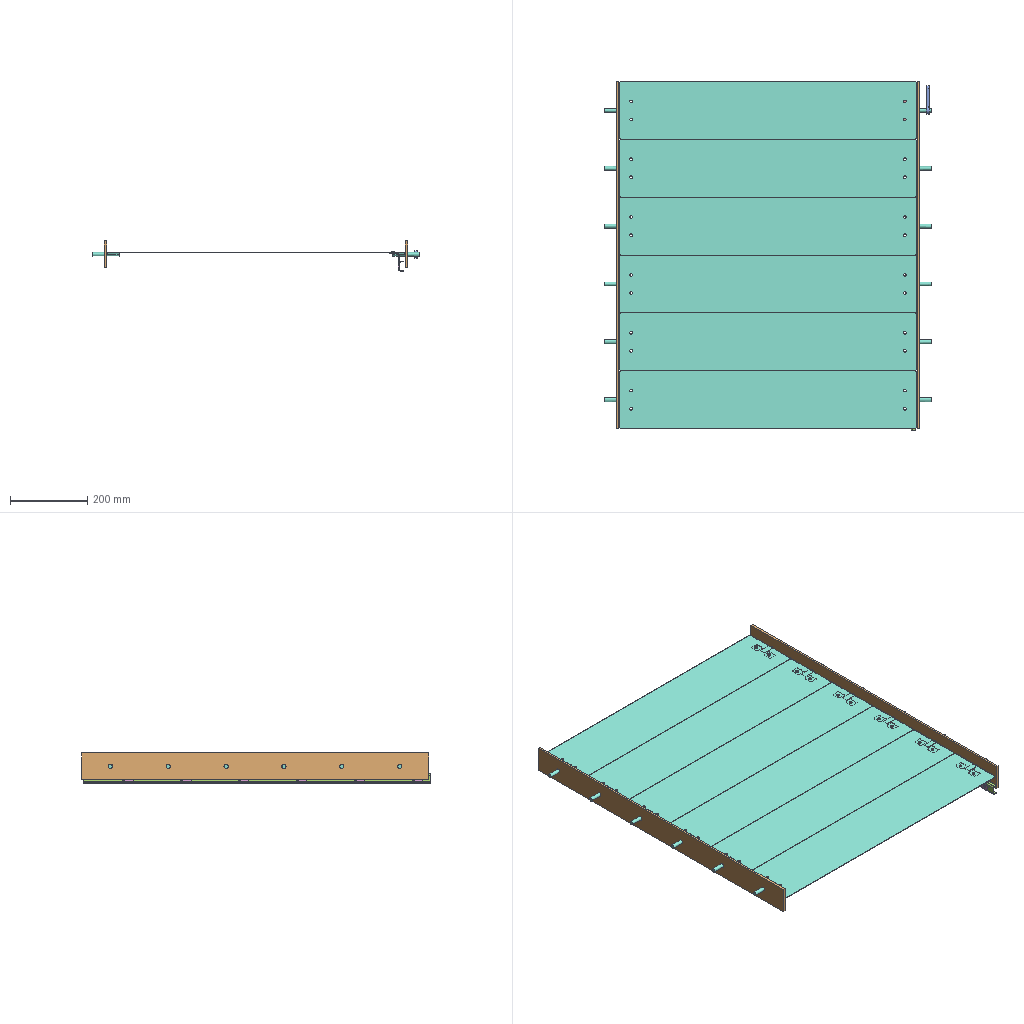Assembly | NX | 6 different items | 18 placed | box 850 x 905 x 79 mm
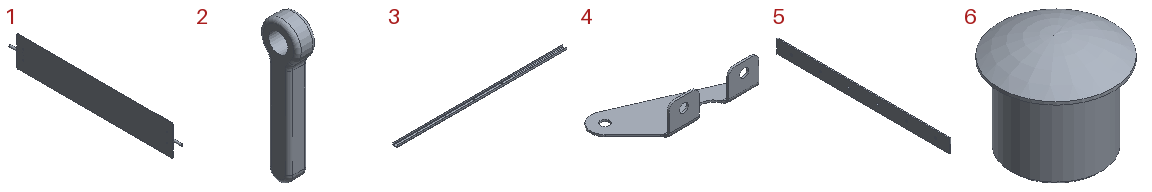Parts list (item | quantity | size | volume | features):
1 | x6 | 10.5 x 850 x 150 mm | 184232 mm3 | features BLEND 3, DATUM_CSYS 3, EXTRUDE 3, SKETCH 2, CPROJ 1
2 | x1 | 10 x 20 x 73.5 mm | 7901 mm3 | features DATUM_CSYS 2, BLEND 1, EXTRUDE 1, SKETCH 1
3 | x1 | 900 x 25 x 12 mm | 46713 mm3 | features SKETCH 4, DATUM_CSYS 3, DATUM_PLANE 2, Flange 2, Base Tab 1, EXTRUDE 1
4 | x6 | 96 x 46 x 24 mm | 4607 mm3 | features SKETCH 4, DATUM_CSYS 3, DATUM_PLANE 2, EXTRUDE 2, Flange 2, BLEND 1, Base Tab 1
5 | x2 | 6 x 900 x 70 mm | 374579 mm3 | features DATUM_CSYS 2, EXTRUDE 1, SKETCH 1
6 | x2 | 8.8 x 8.8 x 7.684 mm | 289.37 mm3 | features DATUM_CSYS 2, CHAMFER 1, SKETCH 1, SWP104 1
Mates (type | each side: item.copy, entity, surface, feature):
Touch | 5.1 face cylinder Extrude(2) | 5.1 face cylinder Extrude(2) | 2 times
Distance | 5.1 face plane Extrude(2) | 5.1 face plane Extrude(2)
Touch | 1.1 face cylinder Extrude(8) | 5.1 face cylinder Extrude(2)
Touch | 1.1 face cylinder Extrude(4) | 5.1 face cylinder Extrude(2) | 2 times
Center22 | 1.1 face plane Extrude(2) | 1.1 face plane Extrude(2) | 5.1 face plane Extrude(2) | 5.1 face plane Extrude(2)
Parallel | 1.1 face plane Extrude(2) | 5.1 face plane Extrude(2)
Fix | assembly component | 2 times
Bond | 1.1 component | assembly component | 6 times
LinearPattern | assembly axis | assembly csys | assembly csys | assembly csys | assembly csys | assembly csys | assembly csys | 2 times
Touch | 4.1 face plane SB Flange(3) | 1.1 face plane Extrude(2)
Touch | 4.1 face cylinder Extrude(5) | 1.1 face cylinder Extrude(2) | 2 times
Bond | 4.1 component | assembly component | 6 times
Touch | 3.1 face cylinder Extrude(6) | 4.1 face cylinder Extrude(6)
Touch | 3.1 face plane SB Tab(2) | 4.1 face plane SB Tab(2)
Parallel | 3.1 face plane SB Flange(3) | 5.1 face plane Extrude(2)
Touch | 4.1 face cylinder Extrude(6) | 3.1 face cylinder Extrude(6)
Touch | 2.1 face cylinder Extrude(2) | 1.1 face cylinder Extrude(4)
Distance | 2.1 face plane Extrude(2) | 1.1 face plane Extrude(4)
Parallel | 2.1 face plane Extrude(2) | 3.1 face plane SB Flange(3)
Touch | 6.1 face cylinder Revolve(2) | 4.1 face cylinder Extrude(5) | 2 times
Touch | 6.1 face plane Revolve(2) | 4.1 face plane SB Flange(4)
Touch | 6.1 face plane Revolve(2) | 4.1 face plane SB Flange(3)